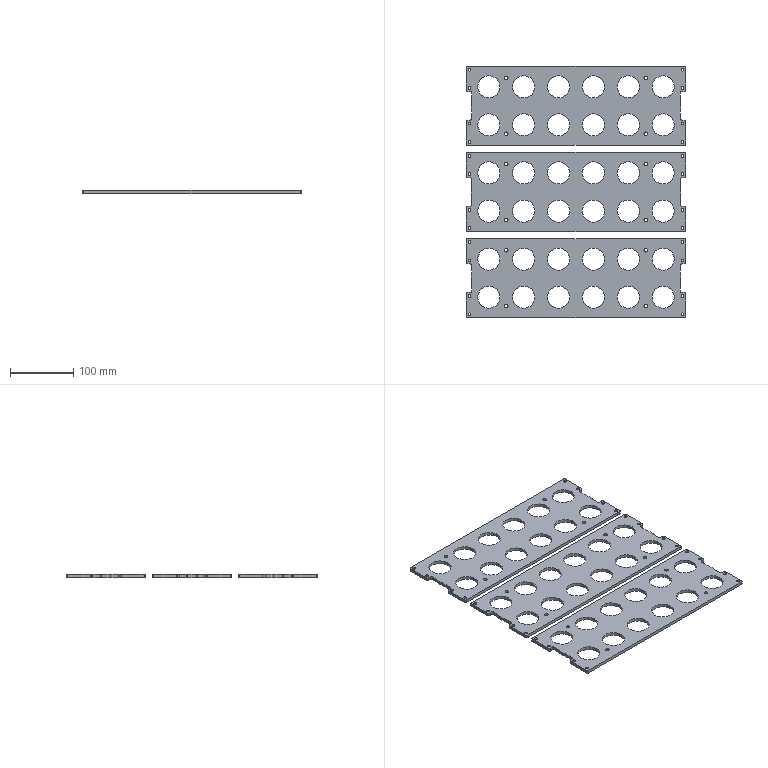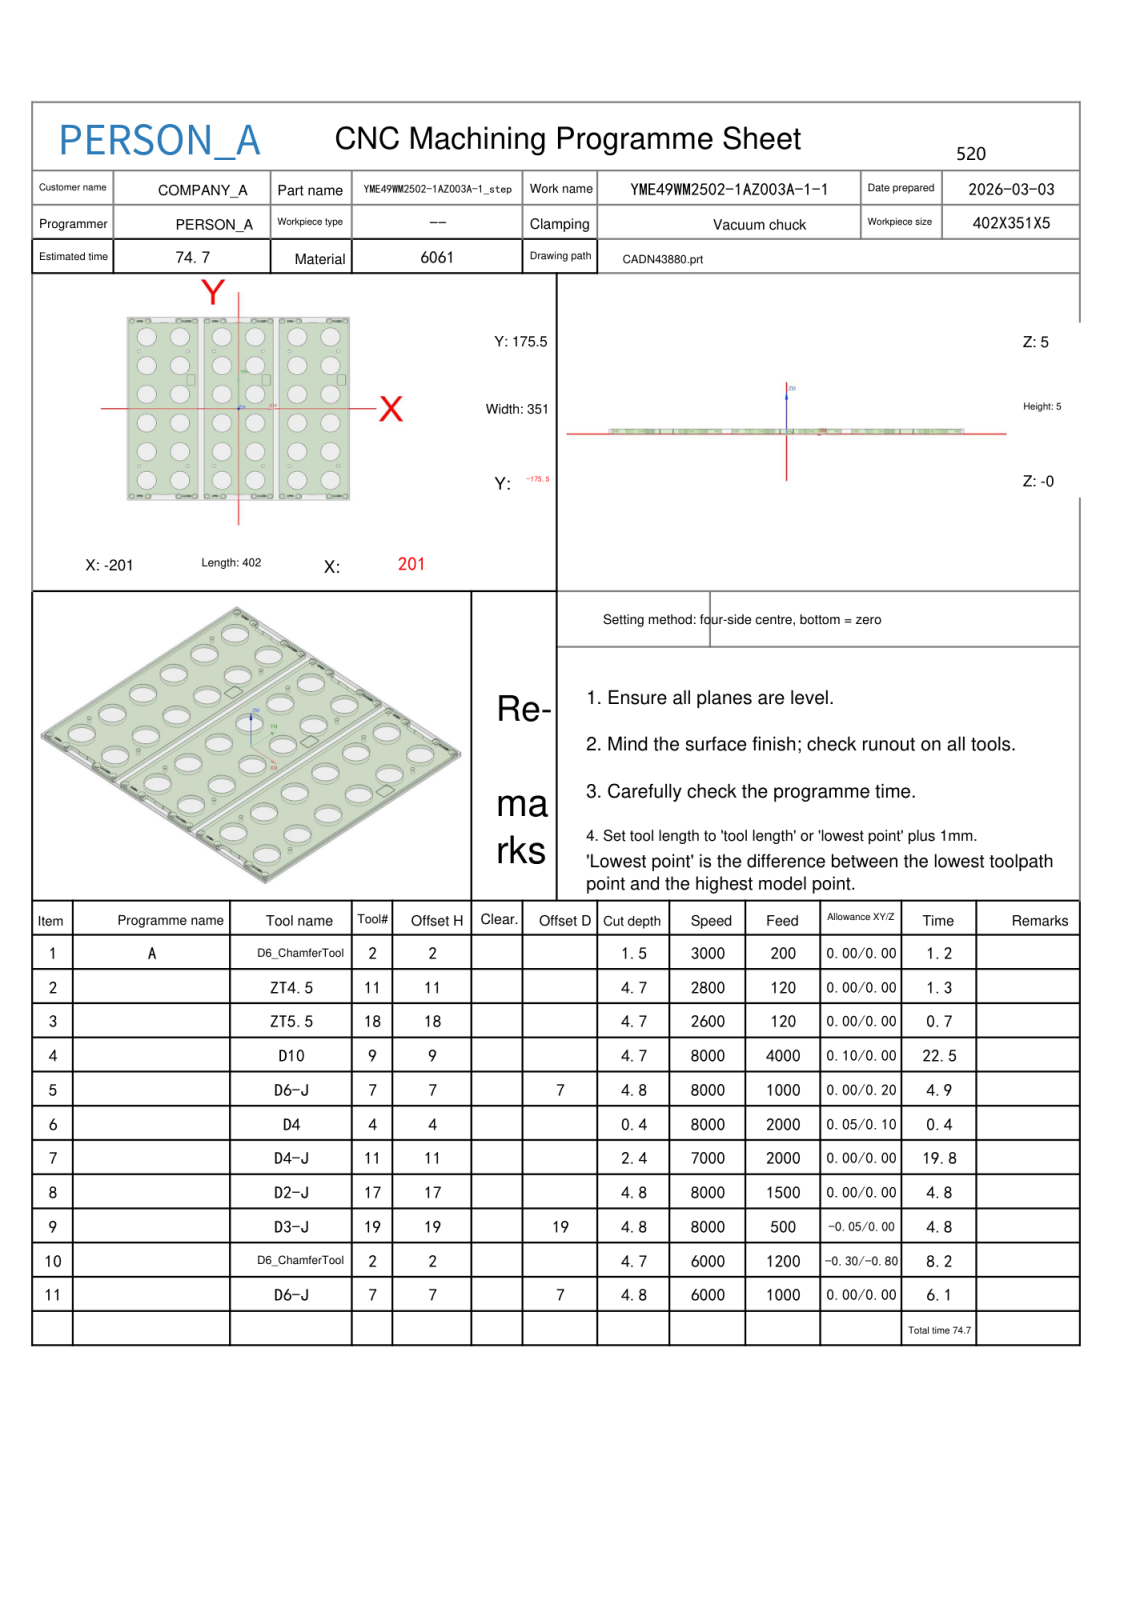NC program | NX | posted by the shop | part box 346 x 397 x 5 mm
Lines 162 to 1032 of 51232:
N4 T09 M06
(D10  D=10. R=0. H=09 ce=0.10 di=0.10)
G00 G90 G54 X166.419 Y-149.9 M03 S8000
G43 H09 Z35.
M08
Z6.
G01 X166.863 Z5.977 F2000.
X169.057 Y-149.548 Z5.86
X171.153 Y-148.812 Z5.744
X173.084 Y-147.714 Z5.627
X174.789 Y-146.289 Z5.511
X176.214 Y-144.584 Z5.395
X177.312 Y-142.653 Z5.278
X178.048 Y-140.557 Z5.162
X178.4 Y-138.363 Z5.045
Y-137.5 Z5.
G03 X166. Y-125.1 Z4.853 I-12.4 J0.0
X153.6 Y-137.5 Z4.706 I0.0 J-12.4
X166. Y-149.9 Z4.559 I12.4 J0.0
X178.4 Y-137.5 Z4.413 I0.0 J12.4
X166. Y-125.1 Z4.266 I-12.4 J0.0
X153.6 Y-137.5 Z4.119 I0.0 J-12.4
X166. Y-149.9 Z3.972 I12.4 J0.0
X178.4 Y-137.5 Z3.825 I0.0 J12.4
X166. Y-125.1 Z3.678 I-12.4 J0.0
X153.6 Y-137.5 Z3.531 I0.0 J-12.4
X166. Y-149.9 Z3.384 I12.4 J0.0
X178.4 Y-137.5 Z3.238 I0.0 J12.4
X166. Y-125.1 Z3.091 I-12.4 J0.0
X153.6 Y-137.5 Z2.944 I0.0 J-12.4
X166. Y-149.9 Z2.797 I12.4 J0.0
X178.4 Y-137.5 Z2.65 I0.0 J12.4
X166. Y-125.1 Z2.503 I-12.4 J0.0
X153.6 Y-137.5 Z2.356 I0.0 J-12.4
X166. Y-149.9 Z2.209 I12.4 J0.0
X178.4 Y-137.5 Z2.063 I0.0 J12.4
X166. Y-125.1 Z1.916 I-12.4 J0.0
X153.6 Y-137.5 Z1.769 I0.0 J-12.4
X166. Y-149.9 Z1.622 I12.4 J0.0
X178.4 Y-137.5 Z1.475 I0.0 J12.4
X166. Y-125.1 Z1.328 I-12.4 J0.0
X153.6 Y-137.5 Z1.181 I0.0 J-12.4
X166. Y-149.9 Z1.034 I12.4 J0.0
X178.4 Y-137.5 Z.888 I0.0 J12.4
X166. Y-125.1 Z.741 I-12.4 J0.0
X153.6 Y-137.5 Z.594 I0.0 J-12.4
X166. Y-149.9 Z.447 I12.4 J0.0
X178.4 Y-137.5 Z.3 I0.0 J12.4
X166. Y-125.1 I-12.4 J0.0
X153.6 Y-137.5 I0.0 J-12.4
X166. Y-149.9 I12.4 J0.0
X178.4 Y-137.5 I0.0 J12.4
X178.394 Y-137.1 I-12.4 J0.0
G01 Z1.3
G00 Z35.
X166.419 Y-94.9
Z6.
G01 X166.863 Z5.977
X169.057 Y-94.548 Z5.86
X171.153 Y-93.812 Z5.744
X173.084 Y-92.714 Z5.627
X174.789 Y-91.289 Z5.511
X176.214 Y-89.584 Z5.395
X177.312 Y-87.653 Z5.278
X178.048 Y-85.557 Z5.162
X178.4 Y-83.363 Z5.045
Y-82.5 Z5.
G03 X166. Y-70.1 Z4.853 I-12.4 J0.0
X153.6 Y-82.5 Z4.706 I0.0 J-12.4
X166. Y-94.9 Z4.559 I12.4 J0.0
X178.4 Y-82.5 Z4.413 I0.0 J12.4
X166. Y-70.1 Z4.266 I-12.4 J0.0
X153.6 Y-82.5 Z4.119 I0.0 J-12.4
X166. Y-94.9 Z3.972 I12.4 J0.0
X178.4 Y-82.5 Z3.825 I0.0 J12.4
X166. Y-70.1 Z3.678 I-12.4 J0.0
X153.6 Y-82.5 Z3.531 I0.0 J-12.4
X166. Y-94.9 Z3.384 I12.4 J0.0
X178.4 Y-82.5 Z3.238 I0.0 J12.4
X166. Y-70.1 Z3.091 I-12.4 J0.0
X153.6 Y-82.5 Z2.944 I0.0 J-12.4
X166. Y-94.9 Z2.797 I12.4 J0.0
X178.4 Y-82.5 Z2.65 I0.0 J12.4
X166. Y-70.1 Z2.503 I-12.4 J0.0
X153.6 Y-82.5 Z2.356 I0.0 J-12.4
X166. Y-94.9 Z2.209 I12.4 J0.0
X178.4 Y-82.5 Z2.063 I0.0 J12.4
X166. Y-70.1 Z1.916 I-12.4 J0.0
X153.6 Y-82.5 Z1.769 I0.0 J-12.4
X166. Y-94.9 Z1.622 I12.4 J0.0
X178.4 Y-82.5 Z1.475 I0.0 J12.4
X166. Y-70.1 Z1.328 I-12.4 J0.0
X153.6 Y-82.5 Z1.181 I0.0 J-12.4
X166. Y-94.9 Z1.034 I12.4 J0.0
X178.4 Y-82.5 Z.888 I0.0 J12.4
X166. Y-70.1 Z.741 I-12.4 J0.0
X153.6 Y-82.5 Z.594 I0.0 J-12.4
X166. Y-94.9 Z.447 I12.4 J0.0
X178.4 Y-82.5 Z.3 I0.0 J12.4
X166. Y-70.1 I-12.4 J0.0
X153.6 Y-82.5 I0.0 J-12.4
X166. Y-94.9 I12.4 J0.0
X178.4 Y-82.5 I0.0 J12.4
X178.394 Y-82.1 I-12.4 J0.0
G01 Z1.3
G00 Z35.
X166.419 Y-39.9
Z6.
G01 X166.863 Z5.977
X169.057 Y-39.548 Z5.86
X171.153 Y-38.812 Z5.744
X173.084 Y-37.714 Z5.627
X174.789 Y-36.289 Z5.511
X176.214 Y-34.584 Z5.395
X177.312 Y-32.653 Z5.278
X178.048 Y-30.557 Z5.162
X178.4 Y-28.363 Z5.045
Y-27.5 Z5.
G03 X166. Y-15.1 Z4.853 I-12.4 J0.0
X153.6 Y-27.5 Z4.706 I0.0 J-12.4
X166. Y-39.9 Z4.559 I12.4 J0.0
X178.4 Y-27.5 Z4.413 I0.0 J12.4
X166. Y-15.1 Z4.266 I-12.4 J0.0
X153.6 Y-27.5 Z4.119 I0.0 J-12.4
X166. Y-39.9 Z3.972 I12.4 J0.0
X178.4 Y-27.5 Z3.825 I0.0 J12.4
X166. Y-15.1 Z3.678 I-12.4 J0.0
X153.6 Y-27.5 Z3.531 I0.0 J-12.4
X166. Y-39.9 Z3.384 I12.4 J0.0
X178.4 Y-27.5 Z3.238 I0.0 J12.4
X166. Y-15.1 Z3.091 I-12.4 J0.0
X153.6 Y-27.5 Z2.944 I0.0 J-12.4
X166. Y-39.9 Z2.797 I12.4 J0.0
X178.4 Y-27.5 Z2.65 I0.0 J12.4
X166. Y-15.1 Z2.503 I-12.4 J0.0
X153.6 Y-27.5 Z2.356 I0.0 J-12.4
X166. Y-39.9 Z2.209 I12.4 J0.0
X178.4 Y-27.5 Z2.063 I0.0 J12.4
X166. Y-15.1 Z1.916 I-12.4 J0.0
X153.6 Y-27.5 Z1.769 I0.0 J-12.4
X166. Y-39.9 Z1.622 I12.4 J0.0
X178.4 Y-27.5 Z1.475 I0.0 J12.4
X166. Y-15.1 Z1.328 I-12.4 J0.0
X153.6 Y-27.5 Z1.181 I0.0 J-12.4
X166. Y-39.9 Z1.034 I12.4 J0.0
X178.4 Y-27.5 Z.888 I0.0 J12.4
X166. Y-15.1 Z.741 I-12.4 J0.0
X153.6 Y-27.5 Z.594 I0.0 J-12.4
X166. Y-39.9 Z.447 I12.4 J0.0
X178.4 Y-27.5 Z.3 I0.0 J12.4
X166. Y-15.1 I-12.4 J0.0
X153.6 Y-27.5 I0.0 J-12.4
X166. Y-39.9 I12.4 J0.0
X178.4 Y-27.5 I0.0 J12.4
X178.394 Y-27.1 I-12.4 J0.0
G01 Z1.3
G00 Z35.
X166.419 Y15.1
Z6.
G01 X166.863 Z5.977
X169.057 Y15.452 Z5.86
X171.153 Y16.188 Z5.744
X173.084 Y17.286 Z5.627
X174.789 Y18.711 Z5.511
X176.214 Y20.416 Z5.395
X177.312 Y22.347 Z5.278
X178.048 Y24.443 Z5.162
X178.4 Y26.637 Z5.045
Y27.5 Z5.
G03 X166. Y39.9 Z4.853 I-12.4 J0.0
X153.6 Y27.5 Z4.706 I0.0 J-12.4
X159.234 Y17.108 Z4.613 I12.4 J0.0
X166. Y15.1 Z4.559 I6.766 J10.392
X178.4 Y27.5 Z4.413 I0.0 J12.4
X166. Y39.9 Z4.266 I-12.4 J0.0
X153.6 Y27.5 Z4.119 I0.0 J-12.4
X159.234 Y17.108 Z4.026 I12.4 J0.0
X166. Y15.1 Z3.972 I6.766 J10.392
X178.4 Y27.5 Z3.825 I0.0 J12.4
X166. Y39.9 Z3.678 I-12.4 J0.0
X153.6 Y27.5 Z3.531 I0.0 J-12.4
X159.234 Y17.108 Z3.438 I12.4 J0.0
X166. Y15.1 Z3.384 I6.766 J10.392
X178.4 Y27.5 Z3.238 I0.0 J12.4
X166. Y39.9 Z3.091 I-12.4 J0.0
X153.6 Y27.5 Z2.944 I0.0 J-12.4
X159.234 Y17.108 Z2.851 I12.4 J0.0
X166. Y15.1 Z2.797 I6.766 J10.392
X178.4 Y27.5 Z2.65 I0.0 J12.4
X166. Y39.9 Z2.503 I-12.4 J0.0
X153.6 Y27.5 Z2.356 I0.0 J-12.4
X159.234 Y17.108 Z2.263 I12.4 J0.0
X166. Y15.1 Z2.209 I6.766 J10.392
X178.4 Y27.5 Z2.063 I0.0 J12.4
X166. Y39.9 Z1.916 I-12.4 J0.0
X153.6 Y27.5 Z1.769 I0.0 J-12.4
X159.234 Y17.108 Z1.676 I12.4 J0.0
X166. Y15.1 Z1.622 I6.766 J10.392
X178.4 Y27.5 Z1.475 I0.0 J12.4
X166. Y39.9 Z1.328 I-12.4 J0.0
X153.6 Y27.5 Z1.181 I0.0 J-12.4
X159.234 Y17.108 Z1.088 I12.4 J0.0
X166. Y15.1 Z1.034 I6.766 J10.392
X178.4 Y27.5 Z.888 I0.0 J12.4
X166. Y39.9 Z.741 I-12.4 J0.0
X153.6 Y27.5 Z.594 I0.0 J-12.4
X159.234 Y17.108 Z.501 I12.4 J0.0
X166. Y15.1 Z.447 I6.766 J10.392
X178.4 Y27.5 Z.3 I0.0 J12.4
X166. Y39.9 I-12.4 J0.0
X153.6 Y27.5 I0.0 J-12.4
X166. Y15.1 I12.4 J0.0
X178.4 Y27.5 I0.0 J12.4
X178.394 Y27.9 I-12.4 J0.0
G01 Z1.3
G00 Z35.
X166.419 Y70.1
Z6.
G01 X166.863 Z5.977
X169.057 Y70.452 Z5.86
X171.153 Y71.188 Z5.744
X173.084 Y72.286 Z5.627
X174.789 Y73.711 Z5.511
X176.214 Y75.416 Z5.395
X177.312 Y77.347 Z5.278
X178.048 Y79.443 Z5.162
X178.4 Y81.637 Z5.045
Y82.5 Z5.
G03 X166. Y94.9 Z4.853 I-12.4 J0.0
X153.6 Y82.5 Z4.706 I0.0 J-12.4
X166. Y70.1 Z4.559 I12.4 J0.0
X178.4 Y82.5 Z4.413 I0.0 J12.4
X166. Y94.9 Z4.266 I-12.4 J0.0
X153.6 Y82.5 Z4.119 I0.0 J-12.4
X166. Y70.1 Z3.972 I12.4 J0.0
X178.4 Y82.5 Z3.825 I0.0 J12.4
X166. Y94.9 Z3.678 I-12.4 J0.0
X153.6 Y82.5 Z3.531 I0.0 J-12.4
X166. Y70.1 Z3.384 I12.4 J0.0
X178.4 Y82.5 Z3.238 I0.0 J12.4
X166. Y94.9 Z3.091 I-12.4 J0.0
X153.6 Y82.5 Z2.944 I0.0 J-12.4
X166. Y70.1 Z2.797 I12.4 J0.0
X178.4 Y82.5 Z2.65 I0.0 J12.4
X166. Y94.9 Z2.503 I-12.4 J0.0
X153.6 Y82.5 Z2.356 I0.0 J-12.4
X166. Y70.1 Z2.209 I12.4 J0.0
X178.4 Y82.5 Z2.063 I0.0 J12.4
X166. Y94.9 Z1.916 I-12.4 J0.0
X153.6 Y82.5 Z1.769 I0.0 J-12.4
X166. Y70.1 Z1.622 I12.4 J0.0
X178.4 Y82.5 Z1.475 I0.0 J12.4
X166. Y94.9 Z1.328 I-12.4 J0.0
X153.6 Y82.5 Z1.181 I0.0 J-12.4
X166. Y70.1 Z1.034 I12.4 J0.0
X178.4 Y82.5 Z.888 I0.0 J12.4
X166. Y94.9 Z.741 I-12.4 J0.0
X153.6 Y82.5 Z.594 I0.0 J-12.4
X166. Y70.1 Z.447 I12.4 J0.0
X178.4 Y82.5 Z.3 I0.0 J12.4
X166. Y94.9 I-12.4 J0.0
X153.6 Y82.5 I0.0 J-12.4
X166. Y70.1 I12.4 J0.0
X178.4 Y82.5 I0.0 J12.4
X178.394 Y82.9 I-12.4 J0.0
G01 Z1.3
G00 Z35.
X166.419 Y125.1
Z6.
G01 X166.863 Z5.977
X169.057 Y125.452 Z5.86
X171.153 Y126.188 Z5.744
X173.084 Y127.286 Z5.627
X174.789 Y128.711 Z5.511
X176.214 Y130.416 Z5.395
X177.312 Y132.347 Z5.278
X178.048 Y134.443 Z5.162
X178.4 Y136.637 Z5.045
Y137.5 Z5.
G03 X166. Y149.9 Z4.853 I-12.4 J0.0
X153.6 Y137.5 Z4.706 I0.0 J-12.4
X159.234 Y127.108 Z4.613 I12.4 J0.0
X166. Y125.1 Z4.559 I6.766 J10.392
X178.4 Y137.5 Z4.413 I0.0 J12.4
X166. Y149.9 Z4.266 I-12.4 J0.0
X153.6 Y137.5 Z4.119 I0.0 J-12.4
X159.234 Y127.108 Z4.026 I12.4 J0.0
X166. Y125.1 Z3.972 I6.766 J10.392
X178.4 Y137.5 Z3.825 I0.0 J12.4
X166. Y149.9 Z3.678 I-12.4 J0.0
X153.6 Y137.5 Z3.531 I0.0 J-12.4
X159.234 Y127.108 Z3.438 I12.4 J0.0
X166. Y125.1 Z3.384 I6.766 J10.392
X178.4 Y137.5 Z3.238 I0.0 J12.4
X166. Y149.9 Z3.091 I-12.4 J0.0
X153.6 Y137.5 Z2.944 I0.0 J-12.4
X159.234 Y127.108 Z2.851 I12.4 J0.0
X166. Y125.1 Z2.797 I6.766 J10.392
X178.4 Y137.5 Z2.65 I0.0 J12.4
X166. Y149.9 Z2.503 I-12.4 J0.0
X153.6 Y137.5 Z2.356 I0.0 J-12.4
X159.234 Y127.108 Z2.263 I12.4 J0.0
X166. Y125.1 Z2.209 I6.766 J10.392
X178.4 Y137.5 Z2.063 I0.0 J12.4
X166. Y149.9 Z1.916 I-12.4 J0.0
X153.6 Y137.5 Z1.769 I0.0 J-12.4
X159.234 Y127.108 Z1.676 I12.4 J0.0
X166. Y125.1 Z1.622 I6.766 J10.392
X178.4 Y137.5 Z1.475 I0.0 J12.4
X166. Y149.9 Z1.328 I-12.4 J0.0
X153.6 Y137.5 Z1.181 I0.0 J-12.4
X159.234 Y127.108 Z1.088 I12.4 J0.0
X166. Y125.1 Z1.034 I6.766 J10.392
X178.4 Y137.5 Z.888 I0.0 J12.4
X166. Y149.9 Z.741 I-12.4 J0.0
X153.6 Y137.5 Z.594 I0.0 J-12.4
X159.234 Y127.108 Z.501 I12.4 J0.0
X166. Y125.1 Z.447 I6.766 J10.392
X178.4 Y137.5 Z.3 I0.0 J12.4
X166. Y149.9 I-12.4 J0.0
X153.6 Y137.5 I0.0 J-12.4
X166. Y125.1 I12.4 J0.0
X178.4 Y137.5 I0.0 J12.4
X178.394 Y137.9 I-12.4 J0.0
G01 Z1.3
G00 Z35.
X93.6 Y-137.919
Z6.
G01 Y-138.363 Z5.977
X93.952 Y-140.557 Z5.86
X94.688 Y-142.653 Z5.744
X95.786 Y-144.584 Z5.627
X97.211 Y-146.289 Z5.511
X98.916 Y-147.714 Z5.395
X100.847 Y-148.812 Z5.278
X102.943 Y-149.548 Z5.162
X105.137 Y-149.9 Z5.045
X106. Z5.
G03 X118.4 Y-137.5 Z4.853 I0.0 J12.4
X106. Y-125.1 Z4.706 I-12.4 J0.0
X93.6 Y-137.5 Z4.559 I0.0 J-12.4
X106. Y-149.9 Z4.413 I12.4 J0.0
X118.4 Y-137.5 Z4.266 I0.0 J12.4
X106. Y-125.1 Z4.119 I-12.4 J0.0
X93.6 Y-137.5 Z3.972 I0.0 J-12.4
X106. Y-149.9 Z3.825 I12.4 J0.0
X118.4 Y-137.5 Z3.678 I0.0 J12.4
X106. Y-125.1 Z3.531 I-12.4 J0.0
X93.6 Y-137.5 Z3.384 I0.0 J-12.4
X106. Y-149.9 Z3.238 I12.4 J0.0
X118.4 Y-137.5 Z3.091 I0.0 J12.4
X106. Y-125.1 Z2.944 I-12.4 J0.0
X93.6 Y-137.5 Z2.797 I0.0 J-12.4
X106. Y-149.9 Z2.65 I12.4 J0.0
X118.4 Y-137.5 Z2.503 I0.0 J12.4
X106. Y-125.1 Z2.356 I-12.4 J0.0
X93.6 Y-137.5 Z2.209 I0.0 J-12.4
X106. Y-149.9 Z2.063 I12.4 J0.0
X118.4 Y-137.5 Z1.916 I0.0 J12.4
X106. Y-125.1 Z1.769 I-12.4 J0.0
X93.6 Y-137.5 Z1.622 I0.0 J-12.4
X106. Y-149.9 Z1.475 I12.4 J0.0
X118.4 Y-137.5 Z1.328 I0.0 J12.4
X106. Y-125.1 Z1.181 I-12.4 J0.0
X93.6 Y-137.5 Z1.034 I0.0 J-12.4
X106. Y-149.9 Z.888 I12.4 J0.0
X118.4 Y-137.5 Z.741 I0.0 J12.4
X106. Y-125.1 Z.594 I-12.4 J0.0
X93.6 Y-137.5 Z.447 I0.0 J-12.4
X106. Y-149.9 Z.3 I12.4 J0.0
X118.4 Y-137.5 I0.0 J12.4
X106. Y-125.1 I-12.4 J0.0
X93.6 Y-137.5 I0.0 J-12.4
X106. Y-149.9 I12.4 J0.0
X106.4 Y-149.894 I0.0 J12.4
G01 Z1.3
G00 Z35.
X93.6 Y-82.919
Z6.
G01 Y-83.363 Z5.977
X93.952 Y-85.557 Z5.86
X94.688 Y-87.653 Z5.744
X95.786 Y-89.584 Z5.627
X97.211 Y-91.289 Z5.511
X98.916 Y-92.714 Z5.395
X100.847 Y-93.812 Z5.278
X102.943 Y-94.548 Z5.162
X105.137 Y-94.9 Z5.045
X106. Z5.
G03 X118.4 Y-82.5 Z4.853 I0.0 J12.4
X106. Y-70.1 Z4.706 I-12.4 J0.0
X93.6 Y-82.5 Z4.559 I0.0 J-12.4
X106. Y-94.9 Z4.413 I12.4 J0.0
X118.4 Y-82.5 Z4.266 I0.0 J12.4
X106. Y-70.1 Z4.119 I-12.4 J0.0
X93.6 Y-82.5 Z3.972 I0.0 J-12.4
X106. Y-94.9 Z3.825 I12.4 J0.0
X118.4 Y-82.5 Z3.678 I0.0 J12.4
X106. Y-70.1 Z3.531 I-12.4 J0.0
X93.6 Y-82.5 Z3.384 I0.0 J-12.4
X106. Y-94.9 Z3.238 I12.4 J0.0
X118.4 Y-82.5 Z3.091 I0.0 J12.4
X106. Y-70.1 Z2.944 I-12.4 J0.0
X93.6 Y-82.5 Z2.797 I0.0 J-12.4
X106. Y-94.9 Z2.65 I12.4 J0.0
X118.4 Y-82.5 Z2.503 I0.0 J12.4
X106. Y-70.1 Z2.356 I-12.4 J0.0
X93.6 Y-82.5 Z2.209 I0.0 J-12.4
X106. Y-94.9 Z2.063 I12.4 J0.0
X118.4 Y-82.5 Z1.916 I0.0 J12.4
X106. Y-70.1 Z1.769 I-12.4 J0.0
X93.6 Y-82.5 Z1.622 I0.0 J-12.4
X106. Y-94.9 Z1.475 I12.4 J0.0
X118.4 Y-82.5 Z1.328 I0.0 J12.4
X106. Y-70.1 Z1.181 I-12.4 J0.0
X93.6 Y-82.5 Z1.034 I0.0 J-12.4
X106. Y-94.9 Z.888 I12.4 J0.0
X118.4 Y-82.5 Z.741 I0.0 J12.4
X106. Y-70.1 Z.594 I-12.4 J0.0
X93.6 Y-82.5 Z.447 I0.0 J-12.4
X106. Y-94.9 Z.3 I12.4 J0.0
X118.4 Y-82.5 I0.0 J12.4
X106. Y-70.1 I-12.4 J0.0
X93.6 Y-82.5 I0.0 J-12.4
X106. Y-94.9 I12.4 J0.0
X106.4 Y-94.894 I0.0 J12.4
G01 Z1.3
G00 Z35.
X106.419 Y-39.9
Z6.
G01 X106.863 Z5.977
X109.057 Y-39.548 Z5.86
X111.153 Y-38.812 Z5.744
X113.084 Y-37.714 Z5.627
X114.789 Y-36.289 Z5.511
X116.214 Y-34.584 Z5.395
X117.312 Y-32.653 Z5.278
X118.048 Y-30.557 Z5.162
X118.4 Y-28.363 Z5.045
Y-27.5 Z5.
G03 X106. Y-15.1 Z4.853 I-12.4 J0.0
X93.6 Y-27.5 Z4.706 I0.0 J-12.4
X106. Y-39.9 Z4.559 I12.4 J0.0
X118.4 Y-27.5 Z4.413 I0.0 J12.4
X106. Y-15.1 Z4.266 I-12.4 J0.0
X93.6 Y-27.5 Z4.119 I0.0 J-12.4
X106. Y-39.9 Z3.972 I12.4 J0.0
X118.4 Y-27.5 Z3.825 I0.0 J12.4
X106. Y-15.1 Z3.678 I-12.4 J0.0
X93.6 Y-27.5 Z3.531 I0.0 J-12.4
X106. Y-39.9 Z3.384 I12.4 J0.0
X118.4 Y-27.5 Z3.238 I0.0 J12.4
X106. Y-15.1 Z3.091 I-12.4 J0.0
X93.6 Y-27.5 Z2.944 I0.0 J-12.4
X106. Y-39.9 Z2.797 I12.4 J0.0
X118.4 Y-27.5 Z2.65 I0.0 J12.4
X106. Y-15.1 Z2.503 I-12.4 J0.0
X93.6 Y-27.5 Z2.356 I0.0 J-12.4
X106. Y-39.9 Z2.209 I12.4 J0.0
X118.4 Y-27.5 Z2.063 I0.0 J12.4
X106. Y-15.1 Z1.916 I-12.4 J0.0
X93.6 Y-27.5 Z1.769 I0.0 J-12.4
X106. Y-39.9 Z1.622 I12.4 J0.0
X118.4 Y-27.5 Z1.475 I0.0 J12.4
X106. Y-15.1 Z1.328 I-12.4 J0.0
X93.6 Y-27.5 Z1.181 I0.0 J-12.4
X106. Y-39.9 Z1.034 I12.4 J0.0
X118.4 Y-27.5 Z.888 I0.0 J12.4
X106. Y-15.1 Z.741 I-12.4 J0.0
X93.6 Y-27.5 Z.594 I0.0 J-12.4
X106. Y-39.9 Z.447 I12.4 J0.0
X118.4 Y-27.5 Z.3 I0.0 J12.4
X106. Y-15.1 I-12.4 J0.0
X93.6 Y-27.5 I0.0 J-12.4
X106. Y-39.9 I12.4 J0.0
X118.4 Y-27.5 I0.0 J12.4
X118.394 Y-27.1 I-12.4 J0.0
G01 Z1.3
G00 Z35.
X106.419 Y15.1
Z6.
G01 X106.863 Z5.977
X109.057 Y15.452 Z5.86
X111.153 Y16.188 Z5.744
X113.084 Y17.286 Z5.627
X114.789 Y18.711 Z5.511
X116.214 Y20.416 Z5.395
X117.312 Y22.347 Z5.278
X118.048 Y24.443 Z5.162
X118.4 Y26.637 Z5.045
Y27.5 Z5.
G03 X106. Y39.9 Z4.853 I-12.4 J0.0
X93.6 Y27.5 Z4.706 I0.0 J-12.4
X106. Y15.1 Z4.559 I12.4 J0.0
X118.4 Y27.5 Z4.413 I0.0 J12.4
X106. Y39.9 Z4.266 I-12.4 J0.0
X93.6 Y27.5 Z4.119 I0.0 J-12.4
X106. Y15.1 Z3.972 I12.4 J0.0
X118.4 Y27.5 Z3.825 I0.0 J12.4
X106. Y39.9 Z3.678 I-12.4 J0.0
X93.6 Y27.5 Z3.531 I0.0 J-12.4
X106. Y15.1 Z3.384 I12.4 J0.0
X118.4 Y27.5 Z3.238 I0.0 J12.4
X106. Y39.9 Z3.091 I-12.4 J0.0
X93.6 Y27.5 Z2.944 I0.0 J-12.4
X106. Y15.1 Z2.797 I12.4 J0.0
X118.4 Y27.5 Z2.65 I0.0 J12.4
X106. Y39.9 Z2.503 I-12.4 J0.0
X93.6 Y27.5 Z2.356 I0.0 J-12.4
X106. Y15.1 Z2.209 I12.4 J0.0
X118.4 Y27.5 Z2.063 I0.0 J12.4
X106. Y39.9 Z1.916 I-12.4 J0.0
X93.6 Y27.5 Z1.769 I0.0 J-12.4
X106. Y15.1 Z1.622 I12.4 J0.0
X118.4 Y27.5 Z1.475 I0.0 J12.4
X106. Y39.9 Z1.328 I-12.4 J0.0
X93.6 Y27.5 Z1.181 I0.0 J-12.4
X106. Y15.1 Z1.034 I12.4 J0.0
X118.4 Y27.5 Z.888 I0.0 J12.4
X106. Y39.9 Z.741 I-12.4 J0.0
X93.6 Y27.5 Z.594 I0.0 J-12.4
X106. Y15.1 Z.447 I12.4 J0.0
X118.4 Y27.5 Z.3 I0.0 J12.4
X106. Y39.9 I-12.4 J0.0
X93.6 Y27.5 I0.0 J-12.4
X106. Y15.1 I12.4 J0.0
X118.4 Y27.5 I0.0 J12.4
X118.394 Y27.9 I-12.4 J0.0
G01 Z1.3
G00 Z35.
X106.419 Y70.1
Z6.
G01 X106.863 Z5.977
X109.057 Y70.452 Z5.86
X111.153 Y71.188 Z5.744
X113.084 Y72.286 Z5.627
X114.789 Y73.711 Z5.511
X116.214 Y75.416 Z5.395
X117.312 Y77.347 Z5.278
X118.048 Y79.443 Z5.162
X118.4 Y81.637 Z5.045
Y82.5 Z5.
G03 X106. Y94.9 Z4.853 I-12.4 J0.0
X93.6 Y82.5 Z4.706 I0.0 J-12.4
X106. Y70.1 Z4.559 I12.4 J0.0
X118.4 Y82.5 Z4.413 I0.0 J12.4
X106. Y94.9 Z4.266 I-12.4 J0.0
X93.6 Y82.5 Z4.119 I0.0 J-12.4
X106. Y70.1 Z3.972 I12.4 J0.0
X118.4 Y82.5 Z3.825 I0.0 J12.4
X106. Y94.9 Z3.678 I-12.4 J0.0
X93.6 Y82.5 Z3.531 I0.0 J-12.4
X106. Y70.1 Z3.384 I12.4 J0.0
X118.4 Y82.5 Z3.238 I0.0 J12.4
X106. Y94.9 Z3.091 I-12.4 J0.0
X93.6 Y82.5 Z2.944 I0.0 J-12.4
X106. Y70.1 Z2.797 I12.4 J0.0
X118.4 Y82.5 Z2.65 I0.0 J12.4
X106. Y94.9 Z2.503 I-12.4 J0.0
X93.6 Y82.5 Z2.356 I0.0 J-12.4
X106. Y70.1 Z2.209 I12.4 J0.0
X118.4 Y82.5 Z2.063 I0.0 J12.4
X106. Y94.9 Z1.916 I-12.4 J0.0
X93.6 Y82.5 Z1.769 I0.0 J-12.4
X106. Y70.1 Z1.622 I12.4 J0.0
X118.4 Y82.5 Z1.475 I0.0 J12.4
X106. Y94.9 Z1.328 I-12.4 J0.0
X93.6 Y82.5 Z1.181 I0.0 J-12.4
X106. Y70.1 Z1.034 I12.4 J0.0
X118.4 Y82.5 Z.888 I0.0 J12.4
X106. Y94.9 Z.741 I-12.4 J0.0
X93.6 Y82.5 Z.594 I0.0 J-12.4
X106. Y70.1 Z.447 I12.4 J0.0
X118.4 Y82.5 Z.3 I0.0 J12.4
X106. Y94.9 I-12.4 J0.0
X93.6 Y82.5 I0.0 J-12.4
X106. Y70.1 I12.4 J0.0
X118.4 Y82.5 I0.0 J12.4
X118.394 Y82.9 I-12.4 J0.0
G01 Z1.3
G00 Z35.
X118.4 Y137.919
Z6.
G01 Y138.363 Z5.977
X118.048 Y140.557 Z5.86
X117.312 Y142.653 Z5.744
X116.214 Y144.584 Z5.627
X114.789 Y146.289 Z5.511
X113.084 Y147.714 Z5.395
X111.153 Y148.812 Z5.278
X109.057 Y149.548 Z5.162
X106.863 Y149.9 Z5.045
X106. Z5.
G03 X93.6 Y137.5 Z4.853 I0.0 J-12.4
X106. Y125.1 Z4.706 I12.4 J0.0
X118.4 Y137.5 Z4.559 I0.0 J12.4
X106. Y149.9 Z4.413 I-12.4 J0.0
X93.6 Y137.5 Z4.266 I0.0 J-12.4
X106. Y125.1 Z4.119 I12.4 J0.0
X118.4 Y137.5 Z3.972 I0.0 J12.4
X106. Y149.9 Z3.825 I-12.4 J0.0
X93.6 Y137.5 Z3.678 I0.0 J-12.4
X106. Y125.1 Z3.531 I12.4 J0.0
X118.4 Y137.5 Z3.384 I0.0 J12.4
X106. Y149.9 Z3.238 I-12.4 J0.0
X93.6 Y137.5 Z3.091 I0.0 J-12.4
X106. Y125.1 Z2.944 I12.4 J0.0
X118.4 Y137.5 Z2.797 I0.0 J12.4
X106. Y149.9 Z2.65 I-12.4 J0.0
X93.6 Y137.5 Z2.503 I0.0 J-12.4
X106. Y125.1 Z2.356 I12.4 J0.0
X118.4 Y137.5 Z2.209 I0.0 J12.4
X106. Y149.9 Z2.063 I-12.4 J0.0
X93.6 Y137.5 Z1.916 I0.0 J-12.4
X106. Y125.1 Z1.769 I12.4 J0.0
X118.4 Y137.5 Z1.622 I0.0 J12.4
X106. Y149.9 Z1.475 I-12.4 J0.0
X93.6 Y137.5 Z1.328 I0.0 J-12.4
X106. Y125.1 Z1.181 I12.4 J0.0
X118.4 Y137.5 Z1.034 I0.0 J12.4
X106. Y149.9 Z.888 I-12.4 J0.0
X93.6 Y137.5 Z.741 I0.0 J-12.4
X106. Y125.1 Z.594 I12.4 J0.0
X118.4 Y137.5 Z.447 I0.0 J12.4
X106. Y149.9 Z.3 I-12.4 J0.0
X93.6 Y137.5 I0.0 J-12.4
X106. Y125.1 I12.4 J0.0
X118.4 Y137.5 I0.0 J12.4
X106. Y149.9 I-12.4 J0.0
X105.6 Y149.894 I0.0 J-12.4
G01 Z1.3
G00 Z35.
X17.6 Y-137.919
Z6.
G01 Y-138.363 Z5.977
X17.952 Y-140.557 Z5.86
X18.688 Y-142.653 Z5.744
X19.786 Y-144.584 Z5.627
X21.211 Y-146.289 Z5.511
X22.916 Y-147.714 Z5.395
X24.847 Y-148.812 Z5.278
X26.943 Y-149.548 Z5.162
X29.137 Y-149.9 Z5.045
X30. Z5.
G03 X42.4 Y-137.5 Z4.853 I0.0 J12.4
X30. Y-125.1 Z4.706 I-12.4 J0.0
X17.6 Y-137.5 Z4.559 I0.0 J-12.4
X30. Y-149.9 Z4.413 I12.4 J0.0
X42.4 Y-137.5 Z4.266 I0.0 J12.4
X30. Y-125.1 Z4.119 I-12.4 J0.0
X17.6 Y-137.5 Z3.972 I0.0 J-12.4
X30. Y-149.9 Z3.825 I12.4 J0.0
X42.4 Y-137.5 Z3.678 I0.0 J12.4
X30. Y-125.1 Z3.531 I-12.4 J0.0
X17.6 Y-137.5 Z3.384 I0.0 J-12.4
X30. Y-149.9 Z3.238 I12.4 J0.0
X42.4 Y-137.5 Z3.091 I0.0 J12.4
X30. Y-125.1 Z2.944 I-12.4 J0.0
X17.6 Y-137.5 Z2.797 I0.0 J-12.4
X30. Y-149.9 Z2.65 I12.4 J0.0
X42.4 Y-137.5 Z2.503 I0.0 J12.4
X30. Y-125.1 Z2.356 I-12.4 J0.0
X17.6 Y-137.5 Z2.209 I0.0 J-12.4
X30. Y-149.9 Z2.063 I12.4 J0.0
X42.4 Y-137.5 Z1.916 I0.0 J12.4
X30. Y-125.1 Z1.769 I-12.4 J0.0
X17.6 Y-137.5 Z1.622 I0.0 J-12.4
X30. Y-149.9 Z1.475 I12.4 J0.0
X42.4 Y-137.5 Z1.328 I0.0 J12.4
X30. Y-125.1 Z1.181 I-12.4 J0.0
X17.6 Y-137.5 Z1.034 I0.0 J-12.4
X30. Y-149.9 Z.888 I12.4 J0.0
X42.4 Y-137.5 Z.741 I0.0 J12.4
X30. Y-125.1 Z.594 I-12.4 J0.0
X17.6 Y-137.5 Z.447 I0.0 J-12.4
X30. Y-149.9 Z.3 I12.4 J0.0
X42.4 Y-137.5 I0.0 J12.4
X30. Y-125.1 I-12.4 J0.0
X17.6 Y-137.5 I0.0 J-12.4
X30. Y-149.9 I12.4 J0.0
X30.4 Y-149.894 I0.0 J12.4
G01 Z1.3
G00 Z35.
X17.6 Y-82.919
Z6.
G01 Y-83.363 Z5.977
X17.952 Y-85.557 Z5.86
X18.688 Y-87.653 Z5.744
X19.786 Y-89.584 Z5.627
X21.211 Y-91.289 Z5.511
X22.916 Y-92.714 Z5.395
X24.847 Y-93.812 Z5.278
X26.943 Y-94.548 Z5.162
X29.137 Y-94.9 Z5.045
X30. Z5.
G03 X42.4 Y-82.5 Z4.853 I0.0 J12.4
X30. Y-70.1 Z4.706 I-12.4 J0.0
X19.608 Y-75.734 Z4.613 I0.0 J-12.4
X17.6 Y-82.5 Z4.559 I10.392 J-6.766
X30. Y-94.9 Z4.413 I12.4 J0.0
X42.4 Y-82.5 Z4.266 I0.0 J12.4
X30. Y-70.1 Z4.119 I-12.4 J0.0
X19.608 Y-75.734 Z4.026 I0.0 J-12.4
X17.6 Y-82.5 Z3.972 I10.392 J-6.766
X30. Y-94.9 Z3.825 I12.4 J0.0
X42.4 Y-82.5 Z3.678 I0.0 J12.4
X30. Y-70.1 Z3.531 I-12.4 J0.0
X19.608 Y-75.734 Z3.438 I0.0 J-12.4
X17.6 Y-82.5 Z3.384 I10.392 J-6.766
X30. Y-94.9 Z3.238 I12.4 J0.0
X42.4 Y-82.5 Z3.091 I0.0 J12.4
X30. Y-70.1 Z2.944 I-12.4 J0.0
X19.608 Y-75.734 Z2.851 I0.0 J-12.4
X17.6 Y-82.5 Z2.797 I10.392 J-6.766
X30. Y-94.9 Z2.65 I12.4 J0.0
X42.4 Y-82.5 Z2.503 I0.0 J12.4
X30. Y-70.1 Z2.356 I-12.4 J0.0
X19.608 Y-75.734 Z2.263 I0.0 J-12.4
X17.6 Y-82.5 Z2.209 I10.392 J-6.766
X30. Y-94.9 Z2.063 I12.4 J0.0
X42.4 Y-82.5 Z1.916 I0.0 J12.4
X30. Y-70.1 Z1.769 I-12.4 J0.0
X19.608 Y-75.734 Z1.676 I0.0 J-12.4
X17.6 Y-82.5 Z1.622 I10.392 J-6.766
X30. Y-94.9 Z1.475 I12.4 J0.0
X42.4 Y-82.5 Z1.328 I0.0 J12.4
X30. Y-70.1 Z1.181 I-12.4 J0.0
X19.608 Y-75.734 Z1.088 I0.0 J-12.4
X17.6 Y-82.5 Z1.034 I10.392 J-6.766
X30. Y-94.9 Z.888 I12.4 J0.0
X42.4 Y-82.5 Z.741 I0.0 J12.4
X30. Y-70.1 Z.594 I-12.4 J0.0
X19.608 Y-75.734 Z.501 I0.0 J-12.4
X17.6 Y-82.5 Z.447 I10.392 J-6.766
X30. Y-94.9 Z.3 I12.4 J0.0
X42.4 Y-82.5 I0.0 J12.4
X30. Y-70.1 I-12.4 J0.0
X17.6 Y-82.5 I0.0 J-12.4
X30. Y-94.9 I12.4 J0.0
X30.4 Y-94.894 I0.0 J12.4
G01 Z1.3
G00 Z35.
X17.6 Y-27.919
Z6.
G01 Y-28.363 Z5.977
X17.952 Y-30.557 Z5.86
X18.688 Y-32.653 Z5.744
X19.786 Y-34.584 Z5.627
X21.211 Y-36.289 Z5.511
X22.916 Y-37.714 Z5.395
X24.847 Y-38.812 Z5.278
X26.943 Y-39.548 Z5.162
X29.137 Y-39.9 Z5.045
X30. Z5.
G03 X42.4 Y-27.5 Z4.853 I0.0 J12.4
X30. Y-15.1 Z4.706 I-12.4 J0.0
X17.6 Y-27.5 Z4.559 I0.0 J-12.4
X30. Y-39.9 Z4.413 I12.4 J0.0
X42.4 Y-27.5 Z4.266 I0.0 J12.4
X30. Y-15.1 Z4.119 I-12.4 J0.0
X17.6 Y-27.5 Z3.972 I0.0 J-12.4
X30. Y-39.9 Z3.825 I12.4 J0.0
X42.4 Y-27.5 Z3.678 I0.0 J12.4
X30. Y-15.1 Z3.531 I-12.4 J0.0
X17.6 Y-27.5 Z3.384 I0.0 J-12.4
X30. Y-39.9 Z3.238 I12.4 J0.0
X42.4 Y-27.5 Z3.091 I0.0 J12.4
X30. Y-15.1 Z2.944 I-12.4 J0.0
X17.6 Y-27.5 Z2.797 I0.0 J-12.4
X30. Y-39.9 Z2.65 I12.4 J0.0
X42.4 Y-27.5 Z2.503 I0.0 J12.4
X30. Y-15.1 Z2.356 I-12.4 J0.0
X17.6 Y-27.5 Z2.209 I0.0 J-12.4
X30. Y-39.9 Z2.063 I12.4 J0.0
X42.4 Y-27.5 Z1.916 I0.0 J12.4
X30. Y-15.1 Z1.769 I-12.4 J0.0
X17.6 Y-27.5 Z1.622 I0.0 J-12.4
X30. Y-39.9 Z1.475 I12.4 J0.0
X42.4 Y-27.5 Z1.328 I0.0 J12.4
X30. Y-15.1 Z1.181 I-12.4 J0.0
X17.6 Y-27.5 Z1.034 I0.0 J-12.4
X30. Y-39.9 Z.888 I12.4 J0.0
X42.4 Y-27.5 Z.741 I0.0 J12.4
X30. Y-15.1 Z.594 I-12.4 J0.0
X17.6 Y-27.5 Z.447 I0.0 J-12.4
X30. Y-39.9 Z.3 I12.4 J0.0
X42.4 Y-27.5 I0.0 J12.4
X30. Y-15.1 I-12.4 J0.0
X17.6 Y-27.5 I0.0 J-12.4
X30. Y-39.9 I12.4 J0.0
X30.4 Y-39.894 I0.0 J12.4
G01 Z1.3
G00 Z35.
X42.4 Y27.919
Z6.
G01 Y28.363 Z5.977
X42.048 Y30.557 Z5.86
X41.312 Y32.653 Z5.744
X40.214 Y34.584 Z5.627
X38.789 Y36.289 Z5.511
X37.084 Y37.714 Z5.395
X35.153 Y38.812 Z5.278
X33.057 Y39.548 Z5.162
X30.863 Y39.9 Z5.045
X30. Z5.
G03 X17.6 Y27.5 Z4.853 I0.0 J-12.4
X30. Y15.1 Z4.706 I12.4 J0.0
X42.4 Y27.5 Z4.559 I0.0 J12.4
X30. Y39.9 Z4.413 I-12.4 J0.0
X17.6 Y27.5 Z4.266 I0.0 J-12.4
X30. Y15.1 Z4.119 I12.4 J0.0
X42.4 Y27.5 Z3.972 I0.0 J12.4
X30. Y39.9 Z3.825 I-12.4 J0.0
X17.6 Y27.5 Z3.678 I0.0 J-12.4
X30. Y15.1 Z3.531 I12.4 J0.0
X42.4 Y27.5 Z3.384 I0.0 J12.4
X30. Y39.9 Z3.238 I-12.4 J0.0
X17.6 Y27.5 Z3.091 I0.0 J-12.4
X30. Y15.1 Z2.944 I12.4 J0.0
X42.4 Y27.5 Z2.797 I0.0 J12.4
X30. Y39.9 Z2.65 I-12.4 J0.0
X17.6 Y27.5 Z2.503 I0.0 J-12.4
X30. Y15.1 Z2.356 I12.4 J0.0
X42.4 Y27.5 Z2.209 I0.0 J12.4
X30. Y39.9 Z2.063 I-12.4 J0.0
X17.6 Y27.5 Z1.916 I0.0 J-12.4
X30. Y15.1 Z1.769 I12.4 J0.0
X42.4 Y27.5 Z1.622 I0.0 J12.4
X30. Y39.9 Z1.475 I-12.4 J0.0
X17.6 Y27.5 Z1.328 I0.0 J-12.4
X30. Y15.1 Z1.181 I12.4 J0.0
X42.4 Y27.5 Z1.034 I0.0 J12.4
X30. Y39.9 Z.888 I-12.4 J0.0
X17.6 Y27.5 Z.741 I0.0 J-12.4
X30. Y15.1 Z.594 I12.4 J0.0
X42.4 Y27.5 Z.447 I0.0 J12.4
X30. Y39.9 Z.3 I-12.4 J0.0
X17.6 Y27.5 I0.0 J-12.4
X30. Y15.1 I12.4 J0.0
X42.4 Y27.5 I0.0 J12.4
X30. Y39.9 I-12.4 J0.0
X29.6 Y39.894 I0.0 J-12.4
G01 Z1.3
G00 Z35.
X42.4 Y82.919
Z6.
G01 Y83.363 Z5.977
X42.048 Y85.557 Z5.86
X41.312 Y87.653 Z5.744
X40.214 Y89.584 Z5.627
X38.789 Y91.289 Z5.511
X37.084 Y92.714 Z5.395
X35.153 Y93.812 Z5.278
X33.057 Y94.548 Z5.162
X30.863 Y94.9 Z5.045
X30. Z5.
G03 X17.6 Y82.5 Z4.853 I0.0 J-12.4
X30. Y70.1 Z4.706 I12.4 J0.0
X42.4 Y82.5 Z4.559 I0.0 J12.4
X30. Y94.9 Z4.413 I-12.4 J0.0
X17.6 Y82.5 Z4.266 I0.0 J-12.4
X30. Y70.1 Z4.119 I12.4 J0.0
X42.4 Y82.5 Z3.972 I0.0 J12.4
X30. Y94.9 Z3.825 I-12.4 J0.0
X17.6 Y82.5 Z3.678 I0.0 J-12.4
X30. Y70.1 Z3.531 I12.4 J0.0
X42.4 Y82.5 Z3.384 I0.0 J12.4
X30. Y94.9 Z3.238 I-12.4 J0.0
X17.6 Y82.5 Z3.091 I0.0 J-12.4
X30. Y70.1 Z2.944 I12.4 J0.0
X42.4 Y82.5 Z2.797 I0.0 J12.4